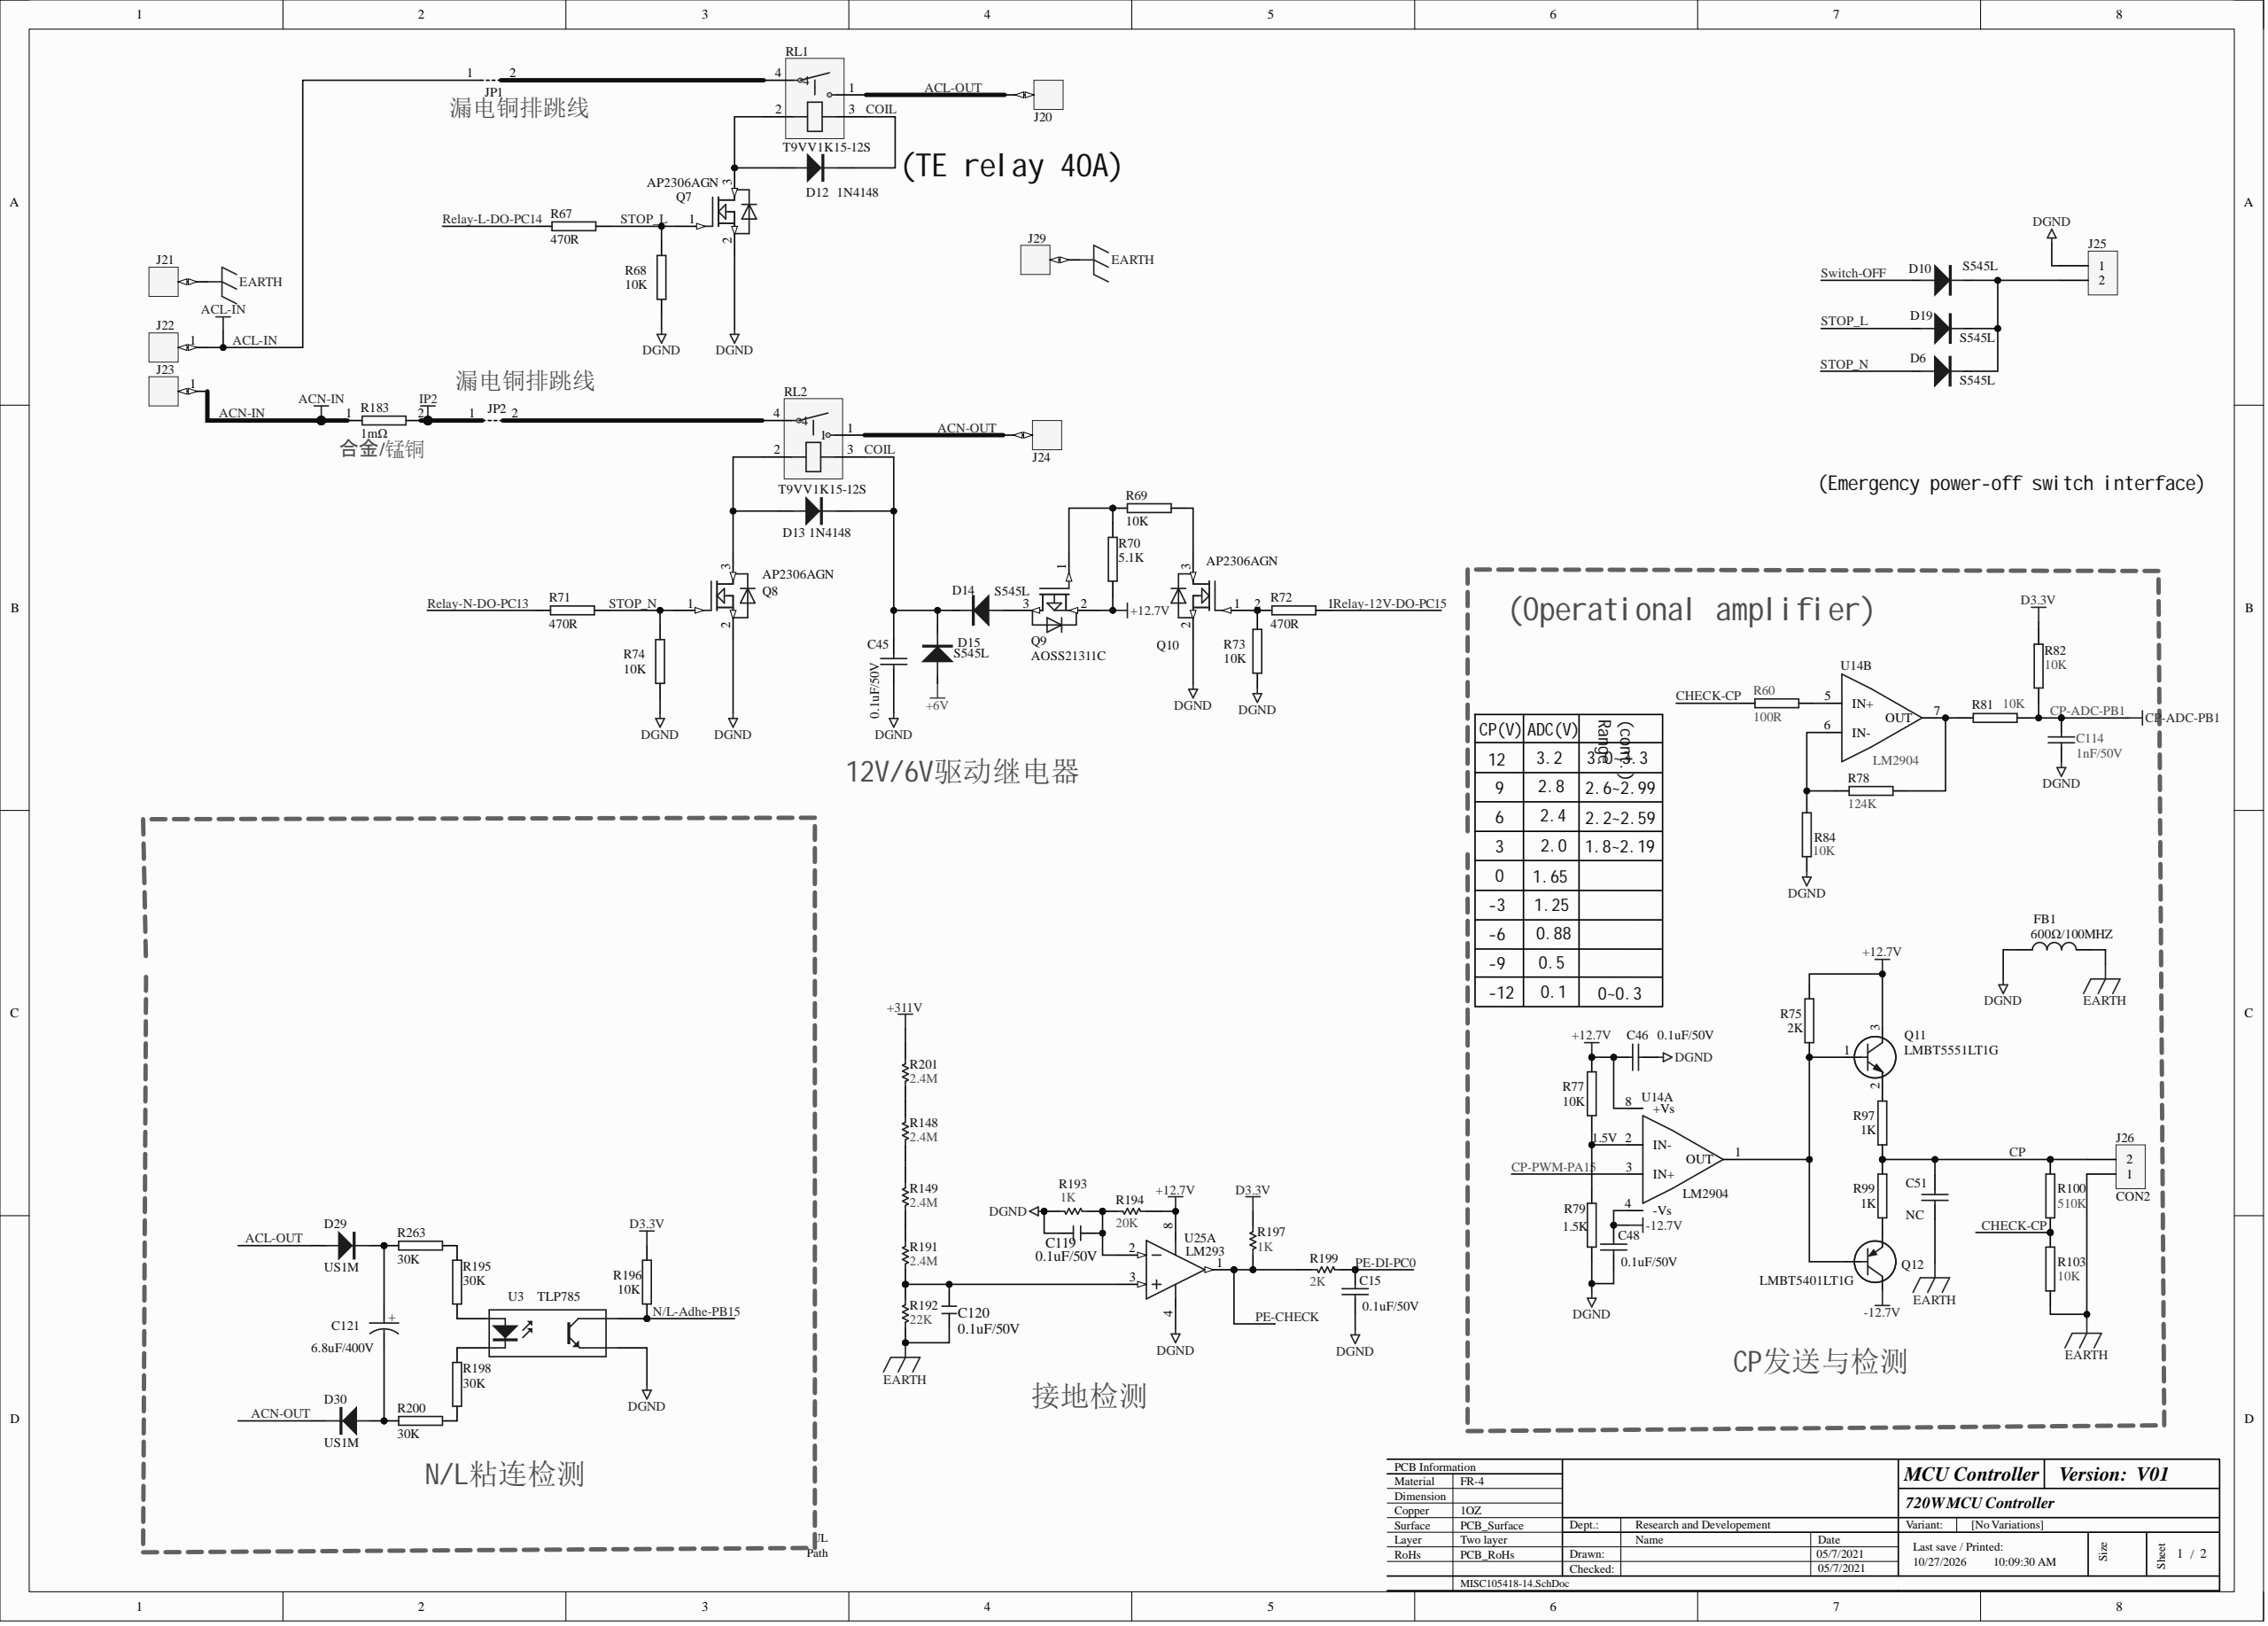Circuit board | Altium Designer | 455 parts | 280 nets | one sheet of the schematic
Parts on this sheet (reference | value | footprint):
C15 | 0.1uF/50V | C0603-T
C45 | 0.1uF/50V | C0805-T
C46 | 0.1uF/50V | C0603-T
C48 | 0.1uF/50V | C0603-T
C51 | NC | C0805-T
C114 | 1nF/50V | C0603-T
C119 | 0.1uF/50V | C0603-T
C120 | 0.1uF/50V | C0603-T
C121 | 6.8uF/400V | CE10-P5.0MM-AI-DS
D6 | S545L | SMA-T
D10 | S545L | SMA-T
D12 | 1N4148 | SOD-123-T
D13 | 1N4148 | SOD-123-T
D14 | S545L | SMA-T
D15 | S545L | SMA-T
D19 | S545L | SMA-T
D29 | US1M | SMA-T
D30 | US1M | SMA-T
FB1 | 600Ω/100MHZ | R1206-T
J20 | Terminal | 接线端子（12X9mm）
J21 | Terminal | 接线端子（12X9mm）
J22 | Terminal | 接线端子（12X9mm）
J23 | Terminal | 接线端子（12X9mm）
J24 | Terminal | 接线端子（12X9mm）
J25 | CON2 | CON2-2.54
J26 | CON2 | CON2-3.81
J29 | Terminal | 接线端子（12X9mm）
JP1 | J* | J0.6-P20.0MM-AI
JP2 | J* | J0.6-P20.0MM-AI
Q7 | AP2306AGN | SOT-23-T
Q8 | AP2306AGN | SOT-23-T
Q9 | AOSS21311C | SOT-23-T
Q10 | AP2306AGN | SOT-23-T
Q11 | LMBT5551LT1G | SOT-23-T
Q12 | LMBT5401LT1G | SOT-23-T
R60 | 100R | R0603-T
R67 | 470R | R0805-T
R68 | 10K | R0805-T
R69 | 10K | R0805-T
R70 | 5.1K | R0805-T
R71 | 470R | R0805-T
R72 | 470R | R0805-T
R73 | 10K | R0805-T
R74 | 10K | R0805-T
R75 | 2K | R0805-T
R77 | 10K | R0603-T
R78 | 124K | R0603-T
R79 | 1.5K | R0603-T
R81 | 10K | R0603-T
R82 | 10K | R0603-T
R84 | 10K | R0603-T
R97 | 1K | R0805-T
R99 | 1K | R0805-T
R100 | 510K | R0805-T
R103 | 10K | R0805-T
R148 | 2.4M | R1206-T
R149 | 2.4M | R1206-T
R183 | 1mΩ | R2512-T
R191 | 2.4M | R1206-T
R192 | 22K | R0805-T
R193 | 1K | R0805-T
R194 | 20K | R0805-T
R195 | 30K | R1206-T
R196 | 10K | R0805-T
R197 | 1K | R0805-T
R198 | 30K | R1206-T
R199 | 2K | R0805-T
R200 | 30K | R1206-T
R201 | 2.4M | R1206-T
R263 | 30K | R1206-T
RL1 | T9VV1K15-12S | 继电器（T9VV1K15-12S）
RL2 | T9VV1K15-12S | 继电器（T9VV1K15-12S）
U3 | TLP785 | OPT-SMT(LTV-817S)
Nets of these parts (net: part-pin ...):
Switch-OFF: D10-1
STOP_N: D6-1 Q8-1 R71-1 R74-2
STOP_L: D19-1 Q7-1 R67-1 R68-2
Relay-N-DO-PC13: R71-2
Relay-L-DO-PC14: R67-2
Relay-12V-DO-PC15: R72-1
PE-DI-PC0: C15-1 R199-1
PE-CHECK: R197-2 R199-2
NetR198_2: R198-2 R200-1
NetR198_1: R198-1 U3-2
NetR195_2: R195-2 U3-1
NetR195_1: R195-1 R263-1
NetR149_1: R149-1 R191-2
NetR148_2: R148-2 R201-1
NetR148_1: R148-1 R149-2
NetR78_2: R78-2 R84-2
NetR78_1: R78-1 R81-2
NetR77_1: R77-1 R79-2
NetR60_1: R60-1
NetQ12_2: Q12-2 R99-2
NetQ11_2: Q11-2 R97-1
NetQ11_1: Q11-1 Q12-1 R75-2
NetQ10_3: Q10-3 R69-1
NetQ10_1: Q10-1 R72-2 R73-2
NetQ9_1: Q9-1 R69-2 R70-2
NetJP2_2: JP2-2 RL2-4
NetJP1_2: JP1-2 RL1-4
NetD14_1: D14-1 Q9-3
NetD13_1: D13-1 Q8-3 RL2-2
NetD12_1: D12-1 Q7-3 RL1-2
NetD6_2: D6-2 D10-2 D19-2 J25-2
NetC121_2: C121-2 D30-1 R200-2
NetC121_1: C121-1 D29-2 R263-2
NetC120_2: C120-2 R191-1 R192-2
NetC119_1: C119-1 R193-1 R194-2
NetC114_1: C114-1 R81-1 R82-2
N/L-Adhe-PB15: R196-1 U3-4
IP2: JP2-1 R183-2
EARTH: C51-2 C120-1 FB1-2 J21-1 J26-1 J29-1 R103-2 R192-1
D3.3V: R82-1 R196-2 R197-1
CP: C51-1 J26-2 R97-2 R99-1 R100-1
COIL: C45-1 D12-2 D13-2 D14-2 D15-2 RL1-3 RL2-3
CHECK-CP: R60-2 R100-2 R103-1
ACN-OUT: D30-2 J24-1 RL2-1
ACN-IN: J23-1 R183-1
ACL-OUT: D29-1 J20-1 RL1-1
ACL-IN: J22-1 JP1-1
-12.7V: C48-1 Q12-3
-: C15-2 C45-2 C46-1 C48-2 C114-2 C119-2 FB1-1 J25-1 Q7-2 Q8-2 Q10-2 R68-1 R73-1 R74-1 R79-1 R84-1 R193-2 U3-3
+311V: R201-2
+12.7V: C46-2 Q9-2 Q11-3 R70-1 R75-1 R77-2 R194-1
+6V: D15-1